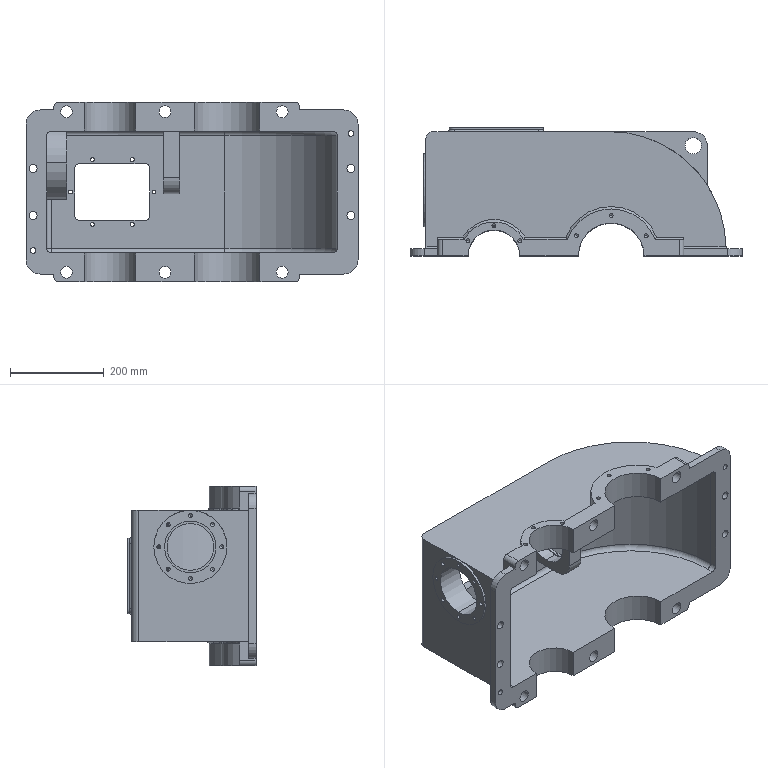Part | SolidWorks | features ICE 13, Fillet 10, HoleWzd 5, MirrorPattern 4, 3DProfileFeature 2, CirPattern 1, Extrusion 1, RevCut 1, Shell 1 | 1 solid | 246 faces | box 708 x 273 x 382 mm | volume 8807514 mm3 | cylinder 142 | plane 53 | cone 40 | torus 10 | sphere 1 | commonest cylinder face diameters 8.5 x52 20 x20 10 x14 25 x12 17 x8 60 x5